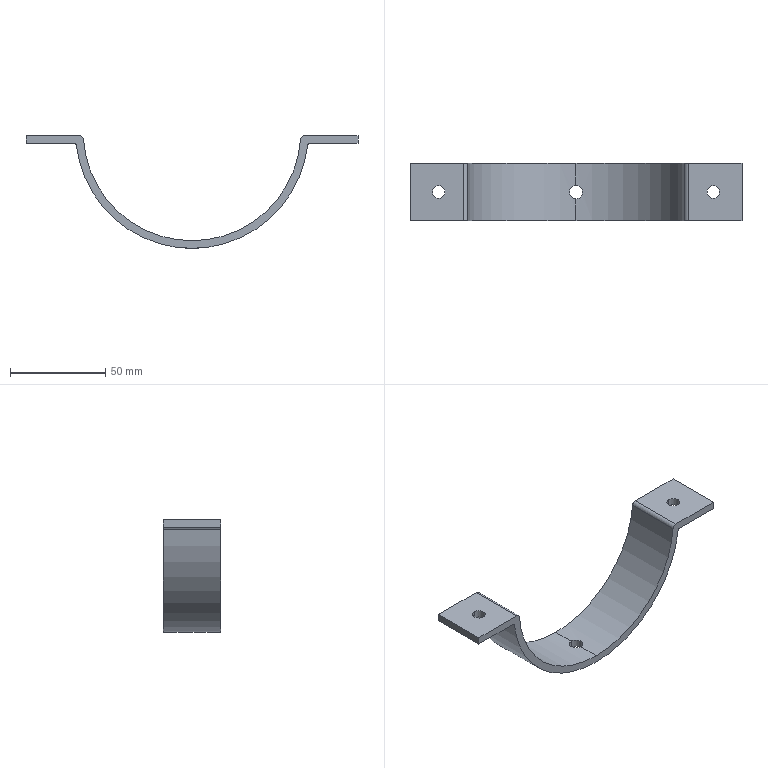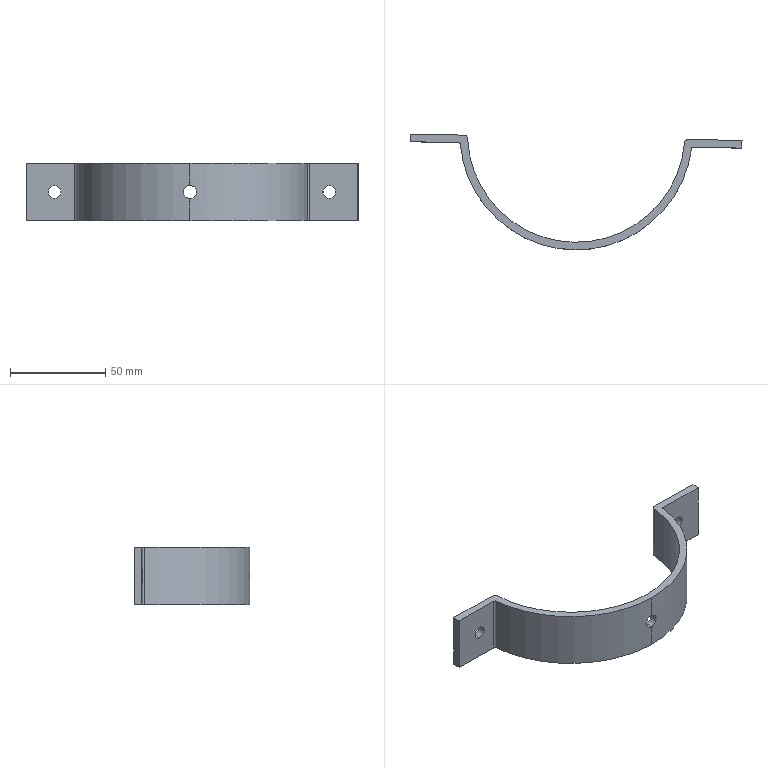Simulation study | abaqus
Set-up summary:
category,name,step,type,value,unit,region
solver,abaqus
solver,version,,,Abaqus/Standard 2020
units,not stated in the deck,,not stated
analysis,deck,,transient,transient
load_step,Step-1,Step-1,transient
load_step,requested,,,1
mesh,nodes,,,6600
mesh,elements,,,6768
element_type,B31,,beam,6768
load,load commands in deck,,count,4
bc,support commands in deck,,count,4
material,MATERIAL-1,,in results
material,MATERIAL-2,,in results
check,setup vs results,,match,"per instance, exact: element labels, types and connectivity; labels of the nodes the elements use; coordinates not compared"
Abaqus input file, long lists of numbers shortened, first 446 of 1701 lines:
*Heading
** Job name: Job-1 Model name: Model-2-Copy-Copy
** Generated by: Abaqus/CAE 2020
*Preprint, echo=NO, model=NO, history=NO, contact=NO
**
** PARTS
**
*Part, name=Part-1
*End Part
**
**
** ASSEMBLY
**
*Assembly, name=Assembly
**
*Instance, name=Part-1-1, part=Part-1
*Node
      1,        3710.,        3000.,        7130.
      2,        3710.,        2700.,        7430.
** (6598 more lines like these left out)
*Element, type=B31
1,   1, 481
2, 481, 482
** (6766 more lines like these left out)
*Nset, nset=Set-1
    7,    9,   10,   16,   27,   29,   30,   36,   47,   49,   50,   56,   72,   75,   77,   78
   92,   95,   97,   98,  112,  115,  117,  118,  132,  135,  137,  138,  152,  155,  157,  158
** (10 more lines like these left out)
*Elset, elset=Set-1
   81,   82,   83,  254,  255,  256,  363,  364,  365,  536,  537,  538,  645,  646,  647,  818
  819,  820, 1031, 1032, 1033, 1107, 1108, 1109, 1313, 1314, 1315, 1389, 1390, 1391, 1595, 1596
** (7 more lines like these left out)
*Nset, nset=Set-3
    7,    9,   10,   16,   27,   29,   30,   36,   47,   49,   50,   56,   72,   75,   77,   78
   92,   95,   97,   98,  112,  115,  117,  118,  132,  135,  137,  138,  152,  155,  157,  158
** (10 more lines like these left out)
*Elset, elset=Set-3
   81,   82,   83,  254,  255,  256,  363,  364,  365,  536,  537,  538,  645,  646,  647,  818
  819,  820, 1031, 1032, 1033, 1107, 1108, 1109, 1313, 1314, 1315, 1389, 1390, 1391, 1595, 1596
** (7 more lines like these left out)
*Nset, nset=Set-4
    7,    9,   10,   16,   27,   29,   30,   36,   47,   49,   50,   56,   72,   75,   77,   78
   92,   95,   97,   98,  112,  115,  117,  118,  132,  135,  137,  138,  152,  155,  157,  158
** (10 more lines like these left out)
*Elset, elset=Set-4
   81,   82,   83,  254,  255,  256,  363,  364,  365,  536,  537,  538,  645,  646,  647,  818
  819,  820, 1031, 1032, 1033, 1107, 1108, 1109, 1313, 1314, 1315, 1389, 1390, 1391, 1595, 1596
** (7 more lines like these left out)
*Nset, nset=Set-5
    7,    8,    9,   10,   16,   17,   18,   20,   27,   28,   29,   30,   36,   37,   38,   40
   47,   48,   49,   50,   56,   57,   58,   60,   72,   74,   75,   76,   77,   78,   79,   80
** (99 more lines like these left out)
*Elset, elset=Set-5
   74,   75,   76,   81,   82,   83,  209,  210,  211,  212,  213,  214,  215,  216,  217,  218
  219,  220,  221,  222,  223,  224,  225,  226,  227,  228,  229,  230,  231,  232,  233,  234
** (97 more lines like these left out)
*Nset, nset=Set-6
    8,    9,   16,   18,   28,   29,   36,   38,   48,   49,   56,   58,   74,   75,   78,   79
   94,   95,   98,   99,  114,  115,  118,  119,  134,  135,  138,  139,  154,  155,  158,  159
** (13 more lines like these left out)
*Elset, elset=Set-6
   77,   78,   79,   80,  257,  258,  259,  260,  359,  360,  361,  362,  539,  540,  541,  542
  641,  642,  643,  644,  821,  822,  823,  824, 1073, 1074, 1075, 1076, 1113, 1114, 1115, 1116
** (10 more lines like these left out)
*Nset, nset=Set-7
    1,    2,    3,    4,    5,    6,    7,    8,    9,   10,   11,   12,   13,   14,   15,   16
   17,   18,   19,   20,   21,   22,   23,   24,   25,   26,   27,   28,   29,   30,   31,   32
** (393 more lines like these left out)
*Elset, elset=Set-7
    5,    6,    7,    8,    9,   10,   11,   12,   13,   14,   15,   16,   17,   18,   19,   20
   21,   22,   23,   24,   25,   26,   27,   28,   29,   30,   31,   32,   33,   34,   35,   36
** (397 more lines like these left out)
*Nset, nset=Set-8
    1,    2,    4,    6,    8,    9,   11,   12,   13,   15,   16,   18,   21,   22,   24,   26
   28,   29,   31,   32,   33,   35,   36,   38,   41,   42,   44,   46,   48,   49,   51,   52
** (28 more lines like these left out)
*Elset, elset=Set-8
    1,    2,    3,    4,   77,   78,   79,   80,  138,  139,  140,  141,  205,  206,  207,  208
  257,  258,  259,  260,  267,  268,  269,  270,  283,  284,  285,  286,  359,  360,  361,  362
** (22 more lines like these left out)
*Nset, nset=Set-9
    1,    2,    3,    4,    5,    6,    7,    8,    9,   10,   11,   12,   13,   14,   15,   16
   17,   18,   19,   20,   21,   22,   23,   24,   25,   26,   27,   28,   29,   30,   31,   32
** (384 more lines like these left out)
*Elset, elset=Set-9
    5,    6,    7,    8,    9,   10,   11,   12,   13,   14,   15,   16,   17,   18,   19,   20
   21,   22,   23,   24,   25,   26,   27,   28,   29,   30,   31,   32,   33,   34,   35,   36
** (385 more lines like these left out)
*Nset, nset=Set-10
    1,    2,    4,    6,    8,    9,   11,   12,   13,   15,   16,   18,   21,   22,   24,   26
   28,   29,   31,   32,   33,   35,   36,   38,   41,   42,   44,   46,   48,   49,   51,   52
** (43 more lines like these left out)
*Elset, elset=Set-10
    1,    2,    3,    4,   77,   78,   79,   80,  138,  139,  140,  141,  205,  206,  207,  208
  257,  258,  259,  260,  267,  268,  269,  270,  283,  284,  285,  286,  359,  360,  361,  362
** (34 more lines like these left out)
*Nset, nset=Set-12
    1,    2,    3,    4,    5,    6,    7,    8,    9,   10,   11,   12,   13,   14,   15,   16
   17,   18,   19,   20,   21,   22,   23,   24,   25,   26,   27,   28,   29,   30,   31,   32
** (262 more lines like these left out)
*Elset, elset=Set-12
    1,    2,    3,    4,    5,    6,    7,   44,   45,   46,   47,   48,   49,   50,   51,   52
   53,   54,   55,   56,   57,   58,   59,   60,   61,   62,   63,   64,   65,   66,   67,   68
** (259 more lines like these left out)
*Nset, nset=Set-13
    1,    4,    8,   12,   13,   16,   21,   24,   28,   32,   33,   36,   41,   44,   48,   52
   53,   56,   61,   64,   68,   71,   74,   78,   81,   84,   88,   91,   94,   98,  101,  104
** (68 more lines like these left out)
*Elset, elset=Set-13
   11,   12,   13,   14,   15,   16,   17,   18,   19,   20,   21,   22,   23,   24,   25,   26
   27,   28,   29,   30,   31,   32,   33,   34,   35,   36,   37,   38,   39,   40,  142,  143
** (66 more lines like these left out)
*Nset, nset=Set-14
    1,    2,    3,    4,    5,    6,    7,    8,    9,   10,   11,   12,   13,   14,   15,   16
   18,   19,   21,   22,   23,   24,   25,   26,   27,   28,   29,   30,   31,   32,   33,   34
** (100 more lines like these left out)
*Elset, elset=Set-14
    1,    2,    3,    4,    8,    9,   10,   11,   12,   13,   14,   15,   16,   17,   18,   19
   20,   21,   22,   23,   24,   25,   26,   27,   28,   29,   30,   31,   32,   33,   34,   35
** (97 more lines like these left out)
*Nset, nset=Set-15
  121,  122,  123,  124,  125,  126,  127,  128,  129,  130,  131,  132,  133,  134,  135,  137
  138,  139,  141,  142,  143,  144,  145,  146,  147,  148,  149,  150,  151,  152,  153,  154
** (100 more lines like these left out)
*Elset, elset=Set-15
 1693, 1694, 1695, 1696, 1700, 1701, 1702, 1703, 1704, 1705, 1706, 1707, 1708, 1709, 1710, 1711
 1712, 1713, 1714, 1715, 1716, 1717, 1718, 1719, 1720, 1721, 1722, 1723, 1724, 1725, 1726, 1727
** (97 more lines like these left out)
*Orientation, name=Ori-1
1., 0., 0., 0., 1., 0.
1, 0.
** Region: (steel:Set-10), (Beam Orientation:Set-14), (Material Orientation:Picked)
*Elset, elset=_I1, internal
    1,    2,    3,    4,   77,   78,   79,   80,  138,  139,  140,  141,  205,  206,  207,  208
  257,  258,  259,  260,  267,  268,  269,  270,  283,  284,  285,  286,  359,  360,  361,  362
** (16 more lines like these left out)
** Section: steel  Profile: Profile-2
*Beam Section, elset=_I1, material=Material-2, temperature=GRADIENTS, section=BOX
40., 28., 2., 2., 2., 2.
1.,0.,0.
** Region: (Section-1:Set-9), (Beam Orientation:Set-12), (Material Orientation:Picked)
*Elset, elset=_I2, internal
    5,    6,    7,   44,   45,   46,   47,   48,   49,   50,   51,   52,   53,   54,   55,   56
   57,   58,   59,   60,   61,   62,   63,   64,   65,   66,   67,   68,   69,   70,   71,   72
** (223 more lines like these left out)
** Section: Section-1  Profile: Profile-1
*Beam Section, elset=_I2, material=Material-1, temperature=GRADIENTS, section=PIPE
55., 12.
0.,0.,-1.
** Region: (Section-1:Set-9), (Beam Orientation:Set-14), (Material Orientation:Picked)
*Elset, elset=_I3, internal
    8,    9,   10,   11,   12,   13,   14,   15,   16,   17,   18,   19,   20,   21,   22,   23
   24,   25,   26,   27,   28,   29,   30,   31,   32,   33,   34,   35,   36,   37,   38,   39
** (79 more lines like these left out)
** Section: Section-1  Profile: Profile-1
*Beam Section, elset=_I3, material=Material-1, temperature=GRADIENTS, section=PIPE
55., 12.
1.,0.,0.
** Region: (steel:Set-10), (Beam Orientation:Set-15), (Material Orientation:Picked)
*Elset, elset=_I4, internal
 1693, 1694, 1695, 1696, 1769, 1770, 1771, 1772, 1803, 1804, 1805, 1806, 1870, 1871, 1872, 1873
 1919, 1920, 1921, 1922, 1959, 1960, 1961, 1962, 1975, 1976, 1977, 1978, 2051, 2052, 2053, 2054
** (16 more lines like these left out)
** Section: steel  Profile: Profile-2
*Beam Section, elset=_I4, material=Material-2, temperature=GRADIENTS, section=BOX
40., 28., 2., 2., 2., 2.
0.,0.,-1.
** Region: (Section-1:Set-9), (Beam Orientation:Set-15), (Material Orientation:Picked)
*Elset, elset=_I5, internal
 1700, 1701, 1702, 1703, 1704, 1705, 1706, 1707, 1708, 1709, 1710, 1711, 1712, 1713, 1714, 1715
 1716, 1717, 1718, 1719, 1720, 1721, 1722, 1723, 1724, 1725, 1726, 1727, 1728, 1729, 1730, 1731
** (79 more lines like these left out)
** Section: Section-1  Profile: Profile-1
*Beam Section, elset=_I5, material=Material-1, temperature=GRADIENTS, section=PIPE
55., 12.
0.,0.,-1.
*End Instance
**
*Nset, nset=Set-1, instance=Part-1-1
  17,  20,  37,  40,  57,  60,  76,  80,  96, 100, 116, 120, 136, 140, 156, 160
 176, 180, 196, 200, 216, 220, 236, 240, 256, 260, 276, 280, 296, 300, 316, 320
** (1 more lines like these left out)
*Nset, nset=Set-2, instance=Part-1-1
  17,  20,  37,  40,  57,  60,  76,  80,  96, 100, 116, 120, 136, 140, 156, 160
 176, 180, 196, 200, 216, 220, 236, 240, 256, 260, 276, 280, 296, 300, 316, 320
** (1 more lines like these left out)
*Nset, nset=Set-58, instance=Part-1-1
   7,  10,  27,  30,  47,  50,  72,  77,  92,  97, 112, 117, 132, 137, 152, 157
 172, 177, 192, 197, 212, 217, 232, 237, 252, 257, 272, 277, 292, 297, 312, 317
** (1 more lines like these left out)
*Nset, nset=Set-59, instance=Part-1-1
   1,   2,   3,   4,   5,   6,   7,   8,   9,  10,  11,  12,  13,  14,  15,  16
  18,  19,  21,  22,  23,  24,  25,  26,  27,  28,  29,  30,  31,  32,  33,  34
** (25 more lines like these left out)
*Nset, nset=m_Set-3, instance=Part-1-1
 205, 223, 243, 305
*Nset, nset=m_Set-6, instance=Part-1-1
 207, 230, 250, 307
*Nset, nset=m_Set-8, instance=Part-1-1
 212, 237, 257, 312
*Nset, nset=m_Set-10, instance=Part-1-1
  72, 412
*Nset, nset=m_Set-12, instance=Part-1-1
  77, 417, 447, 467
*Nset, nset=m_Set-14, instance=Part-1-1
 450, 470
*Nset, nset=m_Set-16, instance=Part-1-1
 137, 172, 297, 352
*Nset, nset=m_Set-18, instance=Part-1-1
  50, 430
*Nset, nset=m_Set-20, instance=Part-1-1
  47, 117, 377, 427
*Nset, nset=m_Set-22, instance=Part-1-1
 112, 372
*Nset, nset=m_Set-24, instance=Part-1-1
 157, 192, 277, 332
*Nset, nset=m_Set-26, instance=Part-1-1
 227, 247
*Nset, nset=m_Set-28, instance=Part-1-1
  45, 110, 370, 425
*Nset, nset=m_Set-30, instance=Part-1-1
   5,  25,  90, 390
*Nset, nset=m_Set-32, instance=Part-1-1
  63, 403, 454, 474
*Nset, nset=m_Set-34, instance=Part-1-1
  70, 410, 445, 465
*Nset, nset=m_Set-36, instance=Part-1-1
 170, 350
*Nset, nset=m_Set-38, instance=Part-1-1
 210, 310
*Nset, nset=m_Set-40, instance=Part-1-1
 130, 167, 290, 347
*Nset, nset=m_Set-42, instance=Part-1-1
 127, 287
*Nset, nset=m_Set-44, instance=Part-1-1
  59, 439
*Nset, nset=m_Set-46, instance=Part-1-1
  54, 103, 363, 434
*Nset, nset=m_Set-48, instance=Part-1-1
 143, 185, 263, 325
*Nset, nset=m_Set-50, instance=Part-1-1
 203, 303
*Nset, nset=m_Set-52, instance=Part-1-1
 225, 245
*Nset, nset=m_Set-54, instance=Part-1-1
 459, 479
*Nset, nset=m_Set-56, instance=Part-1-1
 123, 165, 283, 345
*Nset, nset=s_Set-3, instance=Part-1-1
 385,
*Nset, nset=s_Set-5, instance=Part-1-1
  85, 385
*Nset, nset=s_Set-6, instance=Part-1-1
  87, 387
*Nset, nset=s_Set-8, instance=Part-1-1
  92, 392
*Nset, nset=s_Set-10, instance=Part-1-1
 217, 317
*Nset, nset=s_Set-12, instance=Part-1-1
 197, 337
*Nset, nset=s_Set-14, instance=Part-1-1
 177, 357
*Nset, nset=s_Set-16, instance=Part-1-1
 10, 30
*Nset, nset=s_Set-18, instance=Part-1-1
 132, 292
*Nset, nset=s_Set-20, instance=Part-1-1
 152, 272
*Nset, nset=s_Set-22, instance=Part-1-1
 232, 252
*Nset, nset=s_Set-24, instance=Part-1-1
   7,  27,  97, 397
*Nset, nset=s_Set-26, instance=Part-1-1
 107, 367
*Nset, nset=s_Set-28, instance=Part-1-1
 147, 267
*Nset, nset=s_Set-30, instance=Part-1-1
 150, 187, 270, 327
*Nset, nset=s_Set-32, instance=Part-1-1
 183, 323
*Nset, nset=s_Set-34, instance=Part-1-1
 190, 330
*Nset, nset=s_Set-36, instance=Part-1-1
 443, 463
*Nset, nset=s_Set-38, instance=Part-1-1
  67, 407
*Nset, nset=s_Set-40, instance=Part-1-1
  3, 23
*Nset, nset=s_Set-42, instance=Part-1-1
  43, 423
*Nset, nset=s_Set-44, instance=Part-1-1
 125, 285
*Nset, nset=s_Set-46, instance=Part-1-1
 145, 265
*Nset, nset=s_Set-48, instance=Part-1-1
  14,  34,  83, 383
*Nset, nset=s_Set-50, instance=Part-1-1
  65, 405
*Nset, nset=s_Set-52, instance=Part-1-1
 105, 365
*Nset, nset=s_Set-54, instance=Part-1-1
 163, 343
*Nset, nset=s_Set-56, instance=Part-1-1
 19, 39
*Elset, elset=_m_Surf-1_, internal, instance=Part-1-1, generate
 1923,  1952,     1
*Surface, type=ELEMENT, name=m_Surf-1
_m_Surf-1_,
*Elset, elset=_m_Surf-3_, internal, instance=Part-1-1, generate
 5025,  5054,     1
*Surface, type=ELEMENT, name=m_Surf-3
_m_Surf-3_,
*Elset, elset=_m_Surf-5_, internal, instance=Part-1-1, generate
 1807,  1836,     1
*Surface, type=ELEMENT, name=m_Surf-5
_m_Surf-5_,
*Elset, elset=_m_Surf-7_, internal, instance=Part-1-1, generate
 4909,  4938,     1
*Surface, type=ELEMENT, name=m_Surf-7
_m_Surf-7_,
*Elset, elset=_m_Surf-9_, internal, instance=Part-1-1, generate
 1703,  1732,     1
*Surface, type=ELEMENT, name=m_Surf-9
_m_Surf-9_,
*Elset, elset=_m_Surf-11_, internal, instance=Part-1-1, generate
 4805,  4834,     1
*Surface, type=ELEMENT, name=m_Surf-11
_m_Surf-11_,
*Elset, elset=_m_Surf-13_, internal, instance=Part-1-1, generate
 1985,  2014,     1
*Surface, type=ELEMENT, name=m_Surf-13
_m_Surf-13_,
*Elset, elset=_m_Surf-15_, internal, instance=Part-1-1, generate
 4523,  4552,     1
*Surface, type=ELEMENT, name=m_Surf-15
_m_Surf-15_,
*Elset, elset=_m_Surf-17_, internal, instance=Part-1-1, generate
 3395,  3424,     1
*Surface, type=ELEMENT, name=m_Surf-17
_m_Surf-17_,
*Elset, elset=_m_Surf-19_, internal, instance=Part-1-1, generate
 4241,  4270,     1
*Surface, type=ELEMENT, name=m_Surf-19
_m_Surf-19_,
*Elset, elset=_m_Surf-21_, internal, instance=Part-1-1, generate
 706,  735,    1
*Surface, type=ELEMENT, name=m_Surf-21
_m_Surf-21_,
*Elset, elset=_m_Surf-23_, internal, instance=Part-1-1, generate
 424,  453,    1
*Surface, type=ELEMENT, name=m_Surf-23
_m_Surf-23_,
*Elset, elset=_m_Surf-25_, internal, instance=Part-1-1, generate
 1641,  1670,     1
*Surface, type=ELEMENT, name=m_Surf-25
_m_Surf-25_,
*Elset, elset=_m_Surf-27_, internal, instance=Part-1-1, generate
 773,  802,    1
*Surface, type=ELEMENT, name=m_Surf-27
_m_Surf-27_,
*Elset, elset=_m_Surf-29_, internal, instance=Part-1-1, generate
 1525,  1554,     1
*Surface, type=ELEMENT, name=m_Surf-29
_m_Surf-29_,
*Elset, elset=_m_Surf-31_, internal, instance=Part-1-1, generate
 575,  604,    1
*Surface, type=ELEMENT, name=m_Surf-31
_m_Surf-31_,
*Elset, elset=_m_Surf-33_, internal, instance=Part-1-1, generate
 1421,  1450,     1
*Surface, type=ELEMENT, name=m_Surf-33
_m_Surf-33_,
*Elset, elset=_m_Surf-35_, internal, instance=Part-1-1, generate
 1139,  1168,     1
*Surface, type=ELEMENT, name=m_Surf-35
_m_Surf-35_,
*Elset, elset=_m_Surf-37_, internal, instance=Part-1-1, generate
 5651,  5680,     1
*Surface, type=ELEMENT, name=m_Surf-37
_m_Surf-37_,
*Elset, elset=_m_Surf-39_, internal, instance=Part-1-1, generate
 6346,  6375,     1
*Surface, type=ELEMENT, name=m_Surf-39
_m_Surf-39_,
*Elset, elset=_m_Surf-41_, internal, instance=Part-1-1, generate
 961,  990,    1
*Surface, type=ELEMENT, name=m_Surf-41
_m_Surf-41_,
*Elset, elset=_m_Surf-43_, internal, instance=Part-1-1, generate
 6215,  6244,     1
*Surface, type=ELEMENT, name=m_Surf-43
_m_Surf-43_,
*Elset, elset=_m_Surf-45_, internal, instance=Part-1-1, generate
 1077,  1106,     1
*Surface, type=ELEMENT, name=m_Surf-45
_m_Surf-45_,
*Elset, elset=_m_Surf-47_, internal, instance=Part-1-1, generate
 6413,  6442,     1
*Surface, type=ELEMENT, name=m_Surf-47
_m_Surf-47_,
*Elset, elset=_m_Surf-49_, internal, instance=Part-1-1, generate
 1243,  1272,     1
*Surface, type=ELEMENT, name=m_Surf-49
_m_Surf-49_,
*Elset, elset=_m_Surf-51_, internal, instance=Part-1-1, generate
 293,  322,    1
*Surface, type=ELEMENT, name=m_Surf-51
_m_Surf-51_,
*Elset, elset=_m_Surf-53_, internal, instance=Part-1-1, generate
 1359,  1388,     1
*Surface, type=ELEMENT, name=m_Surf-53
_m_Surf-53_,
*Elset, elset=_m_Surf-55_, internal, instance=Part-1-1, generate
 491,  520,    1
*Surface, type=ELEMENT, name=m_Surf-55
_m_Surf-55_,
*Elset, elset=_m_Surf-57_, internal, instance=Part-1-1, generate
  991,  1017,     1
*Surface, type=ELEMENT, name=m_Surf-57
_m_Surf-57_,
*Elset, elset=_m_Surf-59_, internal, instance=Part-1-1, generate
 4430,  4456,     1
*Surface, type=ELEMENT, name=m_Surf-59
_m_Surf-59_,
*Elset, elset=_m_Surf-61_, internal, instance=Part-1-1, generate
 4743,  4772,     1
*Surface, type=ELEMENT, name=m_Surf-61
_m_Surf-61_,
*Elset, elset=_m_Surf-63_, internal, instance=Part-1-1, generate
 4461,  4490,     1
*Surface, type=ELEMENT, name=m_Surf-63
_m_Surf-63_,
*Elset, elset=_m_Surf-65_, internal, instance=Part-1-1, generate
 3615,  3644,     1
*Surface, type=ELEMENT, name=m_Surf-65
_m_Surf-65_,
*Elset, elset=_m_Surf-67_, internal, instance=Part-1-1, generate
 2935,  2964,     1
*Surface, type=ELEMENT, name=m_Surf-67
_m_Surf-67_,
*Elset, elset=_m_Surf-69_, internal, instance=Part-1-1, generate
 2205,  2234,     1
*Surface, type=ELEMENT, name=m_Surf-69
_m_Surf-69_,
*Elset, elset=_m_Surf-71_, internal, instance=Part-1-1, generate
 4627,  4656,     1
Last 806 lines:
_s_Surf-103_,
*Elset, elset=_s_Surf-105_, internal, instance=Part-1-1, generate
 6033,  6059,     1
*Surface, type=ELEMENT, name=s_Surf-105
_s_Surf-105_,
*Elset, elset=_s_Surf-107_, internal, instance=Part-1-1, generate
 3995,  4021,     1
*Surface, type=ELEMENT, name=s_Surf-107
_s_Surf-107_,
*Elset, elset=_s_Surf-109_, internal, instance=Part-1-1, generate
 5160,  5186,     1
*Surface, type=ELEMENT, name=s_Surf-109
_s_Surf-109_,
*Elset, elset=_s_Surf-111_, internal, instance=Part-1-1, generate
 1494,  1520,     1
*Surface, type=ELEMENT, name=s_Surf-111
_s_Surf-111_,
*Elset, elset=_s_Surf-113_, internal, instance=Part-1-1, generate
 3713,  3739,     1
*Surface, type=ELEMENT, name=s_Surf-113
_s_Surf-113_,
*Elset, elset=_s_Surf-116_, internal, instance=Part-1-1, generate
 6100,  6126,     1
*Surface, type=ELEMENT, name=s_Surf-116
_s_Surf-116_,
*Elset, elset=_s_Surf-118_, internal, instance=Part-1-1, generate
 1610,  1636,     1
*Surface, type=ELEMENT, name=s_Surf-118
_s_Surf-118_,
*Elset, elset=_s_Surf-120_, internal, instance=Part-1-1, generate
 2119,  2145,     1
*Surface, type=ELEMENT, name=s_Surf-120
_s_Surf-120_,
*Elset, elset=_s_Surf-122_, internal, instance=Part-1-1, generate
 5969,  5995,     1
*Surface, type=ELEMENT, name=s_Surf-122
_s_Surf-122_,
*Elset, elset=_s_Surf-124_, internal, instance=Part-1-1, generate
 3431,  3457,     1
*Surface, type=ELEMENT, name=s_Surf-124
_s_Surf-124_,
*Elset, elset=_s_Surf-126_, internal, instance=Part-1-1, generate
 5123,  5149,     1
*Surface, type=ELEMENT, name=s_Surf-126
_s_Surf-126_,
*Elset, elset=_s_Surf-128_, internal, instance=Part-1-1, generate
 4277,  4303,     1
*Surface, type=ELEMENT, name=s_Surf-128
_s_Surf-128_,
*Elset, elset=_s_Surf-130_, internal, instance=Part-1-1, generate
 5405,  5431,     1
*Surface, type=ELEMENT, name=s_Surf-130
_s_Surf-130_,
*Elset, elset=_s_Surf-132_, internal, instance=Part-1-1, generate
 3186,  3212,     1
*Surface, type=ELEMENT, name=s_Surf-132
_s_Surf-132_,
*Elset, elset=_s_Surf-134_, internal, instance=Part-1-1, generate
 5687,  5713,     1
*Surface, type=ELEMENT, name=s_Surf-134
_s_Surf-134_,
*Elset, elset=_s_Surf-136_, internal, instance=Part-1-1, generate
 4314,  4340,     1
*Surface, type=ELEMENT, name=s_Surf-136
_s_Surf-136_,
*Elset, elset=_s_Surf-138_, internal, instance=Part-1-1, generate
 6597,  6623,     1
*Surface, type=ELEMENT, name=s_Surf-138
_s_Surf-138_,
*Elset, elset=_s_Surf-140_, internal, instance=Part-1-1, generate
 2340,  2366,     1
*Surface, type=ELEMENT, name=s_Surf-140
_s_Surf-140_,
*Elset, elset=_s_Surf-142_, internal, instance=Part-1-1, generate
 2303,  2329,     1
*Surface, type=ELEMENT, name=s_Surf-142
_s_Surf-142_,
*Elset, elset=_s_Surf-144_, internal, instance=Part-1-1, generate
 111,  137,    1
*Surface, type=ELEMENT, name=s_Surf-144
_s_Surf-144_,
*Elset, elset=_s_Surf-146_, internal, instance=Part-1-1, generate
 4032,  4058,     1
*Surface, type=ELEMENT, name=s_Surf-146
_s_Surf-146_,
*Elset, elset=_s_Surf-148_, internal, instance=Part-1-1, generate
 5724,  5750,     1
*Surface, type=ELEMENT, name=s_Surf-148
_s_Surf-148_,
*Elset, elset=_s_Surf-150_, internal, instance=Part-1-1, generate
 2622,  2648,     1
*Surface, type=ELEMENT, name=s_Surf-150
_s_Surf-150_,
*Elset, elset=_s_Surf-152_, internal, instance=Part-1-1, generate
 6664,  6690,     1
*Surface, type=ELEMENT, name=s_Surf-152
_s_Surf-152_,
*Elset, elset=_s_Surf-154_, internal, instance=Part-1-1, generate
 4657,  4683,     1
*Surface, type=ELEMENT, name=s_Surf-154
_s_Surf-154_,
*Elset, elset=_s_Surf-156_, internal, instance=Part-1-1, generate
 5558,  5584,     1
*Surface, type=ELEMENT, name=s_Surf-156
_s_Surf-156_,
*Elset, elset=_s_Surf-158_, internal, instance=Part-1-1, generate
 2174,  2200,     1
*Surface, type=ELEMENT, name=s_Surf-158
_s_Surf-158_,
*Elset, elset=_s_Surf-160_, internal, instance=Part-1-1, generate
 2585,  2611,     1
*Surface, type=ELEMENT, name=s_Surf-160
_s_Surf-160_,
*Elset, elset=_s_Surf-162_, internal, instance=Part-1-1, generate
 178,  204,    1
*Surface, type=ELEMENT, name=s_Surf-162
_s_Surf-162_,
*Elset, elset=_s_Surf-164_, internal, instance=Part-1-1, generate
 3750,  3776,     1
*Surface, type=ELEMENT, name=s_Surf-164
_s_Surf-164_,
*Elset, elset=_s_Surf-166_, internal, instance=Part-1-1, generate
 1212,  1238,     1
*Surface, type=ELEMENT, name=s_Surf-166
_s_Surf-166_,
*Elset, elset=_s_Surf-168_, internal, instance=Part-1-1, generate
 2487,  2516,     1
*Surface, type=ELEMENT, name=s_Surf-168
_s_Surf-168_,
*Elset, elset=_s_Surf-170_, internal, instance=Part-1-1, generate
 4179,  4208,     1
*Surface, type=ELEMENT, name=s_Surf-170
_s_Surf-170_,
*Elset, elset=_s_Surf-172_, internal, instance=Part-1-1, generate
 4063,  4092,     1
*Surface, type=ELEMENT, name=s_Surf-172
_s_Surf-172_,
*Elset, elset=_s_Surf-174_, internal, instance=Part-1-1, generate
 2371,  2400,     1
*Surface, type=ELEMENT, name=s_Surf-174
_s_Surf-174_,
*Elset, elset=_s_Surf-176_, internal, instance=Part-1-1, generate
 3959,  3988,     1
*Surface, type=ELEMENT, name=s_Surf-176
_s_Surf-176_,
*Elset, elset=_s_Surf-178_, internal, instance=Part-1-1, generate
 2267,  2296,     1
*Surface, type=ELEMENT, name=s_Surf-178
_s_Surf-178_,
*Elset, elset=_s_Surf-180_, internal, instance=Part-1-1, generate
 3677,  3706,     1
*Surface, type=ELEMENT, name=s_Surf-180
_s_Surf-180_,
*Elset, elset=_s_Surf-182_, internal, instance=Part-1-1, generate
 2549,  2578,     1
*Surface, type=ELEMENT, name=s_Surf-182
_s_Surf-182_,
*Elset, elset=_s_Surf-184_, internal, instance=Part-1-1, generate
 3113,  3142,     1
*Surface, type=ELEMENT, name=s_Surf-184
_s_Surf-184_,
*Elset, elset=_s_Surf-186_, internal, instance=Part-1-1, generate
 2831,  2860,     1
*Surface, type=ELEMENT, name=s_Surf-186
_s_Surf-186_,
*Elset, elset=_s_Surf-188_, internal, instance=Part-1-1, generate
 6064,  6093,     1
*Surface, type=ELEMENT, name=s_Surf-188
_s_Surf-188_,
*Elset, elset=_s_Surf-190_, internal, instance=Part-1-1, generate
 142,  171,    1
*Surface, type=ELEMENT, name=s_Surf-190
_s_Surf-190_,
*Surface, type=NODE, name=m_Set-3_CNS_, internal
m_Set-3, 1.
*Surface, type=NODE, name=s_Set-5_CNS_, internal
s_Set-5, 1.
*Surface, type=NODE, name=m_Set-6_CNS_, internal
m_Set-6, 1.
*Surface, type=NODE, name=s_Set-6_CNS_, internal
s_Set-6, 1.
*Surface, type=NODE, name=m_Set-8_CNS_, internal
m_Set-8, 1.
*Surface, type=NODE, name=s_Set-8_CNS_, internal
s_Set-8, 1.
*Surface, type=NODE, name=m_Set-10_CNS_, internal
m_Set-10, 1.
*Surface, type=NODE, name=s_Set-10_CNS_, internal
s_Set-10, 1.
*Surface, type=NODE, name=m_Set-12_CNS_, internal
m_Set-12, 1.
*Surface, type=NODE, name=s_Set-12_CNS_, internal
s_Set-12, 1.
*Surface, type=NODE, name=m_Set-14_CNS_, internal
m_Set-14, 1.
*Surface, type=NODE, name=s_Set-14_CNS_, internal
s_Set-14, 1.
*Surface, type=NODE, name=m_Set-16_CNS_, internal
m_Set-16, 1.
*Surface, type=NODE, name=s_Set-16_CNS_, internal
s_Set-16, 1.
*Surface, type=NODE, name=m_Set-18_CNS_, internal
m_Set-18, 1.
*Surface, type=NODE, name=s_Set-18_CNS_, internal
s_Set-18, 1.
*Surface, type=NODE, name=m_Set-20_CNS_, internal
m_Set-20, 1.
*Surface, type=NODE, name=s_Set-20_CNS_, internal
s_Set-20, 1.
*Surface, type=NODE, name=m_Set-22_CNS_, internal
m_Set-22, 1.
*Surface, type=NODE, name=s_Set-22_CNS_, internal
s_Set-22, 1.
*Surface, type=NODE, name=m_Set-24_CNS_, internal
m_Set-24, 1.
*Surface, type=NODE, name=s_Set-24_CNS_, internal
s_Set-24, 1.
*Surface, type=NODE, name=m_Set-26_CNS_, internal
m_Set-26, 1.
*Surface, type=NODE, name=s_Set-26_CNS_, internal
s_Set-26, 1.
*Surface, type=NODE, name=m_Set-28_CNS_, internal
m_Set-28, 1.
*Surface, type=NODE, name=s_Set-28_CNS_, internal
s_Set-28, 1.
*Surface, type=NODE, name=m_Set-30_CNS_, internal
m_Set-30, 1.
*Surface, type=NODE, name=s_Set-30_CNS_, internal
s_Set-30, 1.
*Surface, type=NODE, name=m_Set-32_CNS_, internal
m_Set-32, 1.
*Surface, type=NODE, name=s_Set-32_CNS_, internal
s_Set-32, 1.
*Surface, type=NODE, name=m_Set-34_CNS_, internal
m_Set-34, 1.
*Surface, type=NODE, name=s_Set-34_CNS_, internal
s_Set-34, 1.
*Surface, type=NODE, name=m_Set-36_CNS_, internal
m_Set-36, 1.
*Surface, type=NODE, name=s_Set-36_CNS_, internal
s_Set-36, 1.
*Surface, type=NODE, name=m_Set-38_CNS_, internal
m_Set-38, 1.
*Surface, type=NODE, name=s_Set-38_CNS_, internal
s_Set-38, 1.
*Surface, type=NODE, name=m_Set-40_CNS_, internal
m_Set-40, 1.
*Surface, type=NODE, name=s_Set-40_CNS_, internal
s_Set-40, 1.
*Surface, type=NODE, name=m_Set-42_CNS_, internal
m_Set-42, 1.
*Surface, type=NODE, name=s_Set-42_CNS_, internal
s_Set-42, 1.
*Surface, type=NODE, name=m_Set-44_CNS_, internal
m_Set-44, 1.
*Surface, type=NODE, name=s_Set-44_CNS_, internal
s_Set-44, 1.
*Surface, type=NODE, name=m_Set-46_CNS_, internal
m_Set-46, 1.
*Surface, type=NODE, name=s_Set-46_CNS_, internal
s_Set-46, 1.
*Surface, type=NODE, name=m_Set-48_CNS_, internal
m_Set-48, 1.
*Surface, type=NODE, name=s_Set-48_CNS_, internal
s_Set-48, 1.
*Surface, type=NODE, name=m_Set-50_CNS_, internal
m_Set-50, 1.
*Surface, type=NODE, name=s_Set-50_CNS_, internal
s_Set-50, 1.
*Surface, type=NODE, name=m_Set-52_CNS_, internal
m_Set-52, 1.
*Surface, type=NODE, name=s_Set-52_CNS_, internal
s_Set-52, 1.
*Surface, type=NODE, name=m_Set-54_CNS_, internal
m_Set-54, 1.
*Surface, type=NODE, name=s_Set-54_CNS_, internal
s_Set-54, 1.
*Surface, type=NODE, name=m_Set-56_CNS_, internal
m_Set-56, 1.
*Surface, type=NODE, name=s_Set-56_CNS_, internal
s_Set-56, 1.
** Constraint: Constraint-1
*Tie, name=Constraint-1, adjust=yes
s_Surf-170, m_Surf-170
** Constraint: Constraint-2
*Tie, name=Constraint-2, adjust=yes
s_Surf-168, m_Surf-168
** Constraint: Constraint-3
*Tie, name=Constraint-3, adjust=yes
s_Surf-172, m_Surf-172
** Constraint: Constraint-4
*Tie, name=Constraint-4, adjust=yes
s_Surf-174, m_Surf-174
** Constraint: Constraint-5
*Tie, name=Constraint-5, adjust=yes
s_Surf-176, m_Surf-176
** Constraint: Constraint-6
*Tie, name=Constraint-6, adjust=yes
s_Surf-178, m_Surf-178
** Constraint: Constraint-7
*Tie, name=Constraint-7, adjust=yes
s_Surf-180, m_Surf-180
** Constraint: Constraint-8
*Tie, name=Constraint-8, adjust=yes
s_Surf-182, m_Surf-182
** Constraint: Constraint-9
*Tie, name=Constraint-9, adjust=yes
s_Surf-184, m_Surf-184
** Constraint: Constraint-10
*Tie, name=Constraint-10, adjust=yes
s_Surf-186, m_Surf-186
** Constraint: Constraint-11
*Tie, name=Constraint-11, adjust=yes
s_Surf-188, m_Surf-188
** Constraint: Constraint-12
*Tie, name=Constraint-12, adjust=yes
s_Surf-190, m_Surf-190
** Constraint: Constraint-13-node
*Tie, name=Constraint-13-node, adjust=yes
s_Set-5_CNS_, m_Set-3_CNS_
** Constraint: Constraint-14
*Tie, name=Constraint-14, adjust=yes
s_Set-6_CNS_, m_Set-6_CNS_
** Constraint: Constraint-15
*Tie, name=Constraint-15, adjust=yes
s_Set-8_CNS_, m_Set-8_CNS_
** Constraint: Constraint-16
*Tie, name=Constraint-16, adjust=yes
s_Set-10_CNS_, m_Set-10_CNS_
** Constraint: Constraint-17
*Tie, name=Constraint-17, adjust=yes
s_Set-12_CNS_, m_Set-12_CNS_
** Constraint: Constraint-18
*Tie, name=Constraint-18, adjust=yes
s_Set-14_CNS_, m_Set-14_CNS_
** Constraint: Constraint-19
*Tie, name=Constraint-19, adjust=yes
s_Set-16_CNS_, m_Set-16_CNS_
** Constraint: Constraint-20
*Tie, name=Constraint-20, adjust=yes
s_Set-18_CNS_, m_Set-18_CNS_
** Constraint: Constraint-21
*Tie, name=Constraint-21, adjust=yes
s_Set-20_CNS_, m_Set-20_CNS_
** Constraint: Constraint-22
*Tie, name=Constraint-22, adjust=yes
s_Set-22_CNS_, m_Set-22_CNS_
** Constraint: Constraint-23
*Tie, name=Constraint-23, adjust=yes
s_Set-24_CNS_, m_Set-24_CNS_
** Constraint: Constraint-24
*Tie, name=Constraint-24, adjust=yes
s_Set-26_CNS_, m_Set-26_CNS_
** Constraint: Constraint-25
*Tie, name=Constraint-25, adjust=yes
s_Set-28_CNS_, m_Set-28_CNS_
** Constraint: Constraint-26
*Tie, name=Constraint-26, adjust=yes
s_Set-30_CNS_, m_Set-30_CNS_
** Constraint: Constraint-27
*Tie, name=Constraint-27, adjust=yes
s_Set-32_CNS_, m_Set-32_CNS_
** Constraint: Constraint-28
*Tie, name=Constraint-28, adjust=yes
s_Set-34_CNS_, m_Set-34_CNS_
** Constraint: Constraint-29
*Tie, name=Constraint-29, adjust=yes
s_Set-36_CNS_, m_Set-36_CNS_
** Constraint: Constraint-30
*Tie, name=Constraint-30, adjust=yes
s_Set-38_CNS_, m_Set-38_CNS_
** Constraint: Constraint-31
*Tie, name=Constraint-31, adjust=yes
s_Set-40_CNS_, m_Set-40_CNS_
** Constraint: Constraint-32
*Tie, name=Constraint-32, adjust=yes
s_Set-42_CNS_, m_Set-42_CNS_
** Constraint: Constraint-33
*Tie, name=Constraint-33, adjust=yes
s_Set-44_CNS_, m_Set-44_CNS_
** Constraint: Constraint-34
*Tie, name=Constraint-34, adjust=yes
s_Set-46_CNS_, m_Set-46_CNS_
** Constraint: Constraint-35
*Tie, name=Constraint-35, adjust=yes
s_Set-48_CNS_, m_Set-48_CNS_
** Constraint: Constraint-36
*Tie, name=Constraint-36, adjust=yes
s_Set-50_CNS_, m_Set-50_CNS_
** Constraint: Constraint-37
*Tie, name=Constraint-37, adjust=yes
s_Set-52_CNS_, m_Set-52_CNS_
** Constraint: Constraint-38
*Tie, name=Constraint-38, adjust=yes
s_Set-54_CNS_, m_Set-54_CNS_
** Constraint: Constraint-39
*Tie, name=Constraint-39, adjust=yes
s_Set-56_CNS_, m_Set-56_CNS_
** Constraint: Constraint-40
*Tie, name=Constraint-40, adjust=yes
s_Surf-25, m_Surf-25
** Constraint: Constraint-41
*Tie, name=Constraint-41, adjust=yes
s_Surf-27, m_Surf-27
** Constraint: Constraint-42
*Tie, name=Constraint-42, adjust=yes
s_Surf-29, m_Surf-29
** Constraint: Constraint-43
*Tie, name=Constraint-43, adjust=yes
s_Surf-31, m_Surf-31
** Constraint: Constraint-44
*Tie, name=Constraint-44, adjust=yes
s_Surf-33, m_Surf-33
** Constraint: Constraint-45
*Tie, name=Constraint-45, adjust=yes
s_Surf-35, m_Surf-35
** Constraint: Constraint-46
*Tie, name=Constraint-46, adjust=yes
s_Surf-37, m_Surf-37
** Constraint: Constraint-47
*Tie, name=Constraint-47, adjust=yes
s_Surf-39, m_Surf-39
** Constraint: Constraint-48
*Tie, name=Constraint-48, adjust=yes
s_Surf-41, m_Surf-41
** Constraint: Constraint-49
*Tie, name=Constraint-49, adjust=yes
s_Surf-43, m_Surf-43
** Constraint: Constraint-50
*Tie, name=Constraint-50, adjust=yes
s_Surf-45, m_Surf-45
** Constraint: Constraint-51
*Tie, name=Constraint-51, adjust=yes
s_Surf-47, m_Surf-47
** Constraint: Constraint-52
*Tie, name=Constraint-52, adjust=yes
s_Surf-49, m_Surf-49
** Constraint: Constraint-53
*Tie, name=Constraint-53, adjust=yes
s_Surf-51, m_Surf-51
** Constraint: Constraint-54
*Tie, name=Constraint-54, adjust=yes
s_Surf-53, m_Surf-53
** Constraint: Constraint-55
*Tie, name=Constraint-55, adjust=yes
s_Surf-55, m_Surf-55
** Constraint: Constraint-56
*Tie, name=Constraint-56, adjust=yes
s_Surf-57, m_Surf-57
** Constraint: Constraint-57
*Tie, name=Constraint-57, adjust=yes
s_Surf-59, m_Surf-59
** Constraint: Constraint-58
*Tie, name=Constraint-58, adjust=yes
s_Surf-61, m_Surf-61
** Constraint: Constraint-59
*Tie, name=Constraint-59, adjust=yes
s_Surf-63, m_Surf-63
** Constraint: Constraint-60
*Tie, name=Constraint-60, adjust=yes
s_Surf-65, m_Surf-65
** Constraint: Constraint-61
*Tie, name=Constraint-61, adjust=yes
s_Surf-67, m_Surf-67
** Constraint: Constraint-62
*Tie, name=Constraint-62, adjust=yes
s_Surf-69, m_Surf-69
** Constraint: Constraint-63
*Tie, name=Constraint-63, adjust=yes
s_Surf-71, m_Surf-71
** Constraint: Constraint-64
*Tie, name=Constraint-64, adjust=yes
s_Surf-73, m_Surf-73
** Constraint: Constraint-65
*Tie, name=Constraint-65, adjust=yes
s_Surf-75, m_Surf-75
** Constraint: Constraint-66
*Tie, name=Constraint-66, adjust=yes
s_Surf-77, m_Surf-77
** Constraint: Constraint-67
*Tie, name=Constraint-67, adjust=yes
s_Surf-79, m_Surf-79
** Constraint: Constraint-68
*Tie, name=Constraint-68, adjust=yes
s_Surf-81, m_Surf-81
** Constraint: Constraint-69
*Tie, name=Constraint-69, adjust=yes
s_Surf-83, m_Surf-83
** Constraint: Constraint-70
*Tie, name=Constraint-70, adjust=yes
s_Surf-85, m_Surf-85
** Constraint: Constraint-71
*Tie, name=Constraint-71, adjust=yes
s_Surf-87, m_Surf-87
** Constraint: Constraint-72
*Tie, name=Constraint-72, adjust=yes
s_Surf-89, m_Surf-89
** Constraint: Constraint-73
*Tie, name=Constraint-73, adjust=yes
s_Surf-91, m_Surf-91
** Constraint: Constraint-74
*Tie, name=Constraint-74, adjust=yes
s_Surf-93, m_Surf-93
** Constraint: Constraint-75
*Tie, name=Constraint-75, adjust=yes
s_Surf-95, m_Surf-95
** Constraint: Constraint-76
*Tie, name=Constraint-76, adjust=yes
s_Surf-97, m_Surf-97
** Constraint: Constraint-77
*Tie, name=Constraint-77, adjust=yes
s_Surf-99, m_Surf-99
** Constraint: Constraint-78
*Tie, name=Constraint-78, adjust=yes
s_Surf-101, m_Surf-101
** Constraint: Constraint-79
*Tie, name=Constraint-79, adjust=yes
s_Surf-103, m_Surf-103
** Constraint: Constraint-80
*Tie, name=Constraint-80, adjust=yes
s_Surf-105, m_Surf-105
** Constraint: Constraint-81
*Tie, name=Constraint-81, adjust=yes
s_Surf-107, m_Surf-107
** Constraint: Constraint-82
*Tie, name=Constraint-82, adjust=yes
s_Surf-116, m_Surf-115
** Constraint: Constraint-83
*Tie, name=Constraint-83, adjust=yes
s_Surf-111, m_Surf-117
** Constraint: Constraint-84
*Tie, name=Constraint-84, adjust=yes
s_Surf-113, m_Surf-113
** Constraint: Constraint-85
*Tie, name=Constraint-85, adjust=yes
s_Surf-118, m_Surf-118
** Constraint: Constraint-86
*Tie, name=Constraint-86, adjust=yes
s_Surf-120, m_Surf-120
** Constraint: Constraint-87
*Tie, name=Constraint-87, adjust=yes
s_Surf-122, m_Surf-122
** Constraint: Constraint-88
*Tie, name=Constraint-88, adjust=yes
s_Surf-124, m_Surf-124
** Constraint: Constraint-89
*Tie, name=Constraint-89, adjust=yes
s_Surf-126, m_Surf-126
** Constraint: Constraint-90
*Tie, name=Constraint-90, adjust=yes
s_Surf-128, m_Surf-128
** Constraint: Constraint-91
*Tie, name=Constraint-91, adjust=yes
s_Surf-130, m_Surf-130
** Constraint: Constraint-92
*Tie, name=Constraint-92, adjust=yes
s_Surf-132, m_Surf-132
** Constraint: Constraint-93
*Tie, name=Constraint-93, adjust=yes
s_Surf-134, m_Surf-134
** Constraint: Constraint-94
*Tie, name=Constraint-94, adjust=yes
s_Surf-136, m_Surf-136
** Constraint: Constraint-95
*Tie, name=Constraint-95, adjust=yes
s_Surf-138, m_Surf-138
** Constraint: Constraint-96
*Tie, name=Constraint-96, adjust=yes
s_Surf-140, m_Surf-140
** Constraint: Constraint-97
*Tie, name=Constraint-97, adjust=yes
s_Surf-142, m_Surf-142
** Constraint: Constraint-98
*Tie, name=Constraint-98, adjust=yes
s_Surf-144, m_Surf-144
** Constraint: Constraint-99
*Tie, name=Constraint-99, adjust=yes
s_Surf-146, m_Surf-146
** Constraint: Constraint-100
*Tie, name=Constraint-100, adjust=yes
s_Surf-148, m_Surf-148
** Constraint: Constraint-101
*Tie, name=Constraint-101, adjust=yes
s_Surf-150, m_Surf-150
** Constraint: Constraint-102
*Tie, name=Constraint-102, adjust=yes
s_Surf-152, m_Surf-152
** Constraint: Constraint-103
*Tie, name=Constraint-103, adjust=yes
s_Surf-154, m_Surf-154
** Constraint: Constraint-104
*Tie, name=Constraint-104, adjust=yes
s_Surf-156, m_Surf-156
** Constraint: Constraint-105
*Tie, name=Constraint-105, adjust=yes
s_Surf-158, m_Surf-158
** Constraint: Constraint-106
*Tie, name=Constraint-106, adjust=yes
s_Surf-160, m_Surf-160
** Constraint: Constraint-107
*Tie, name=Constraint-107, adjust=yes
s_Surf-162, m_Surf-162
** Constraint: Constraint-108
*Tie, name=Constraint-108, adjust=yes
s_Surf-164, m_Surf-164
** Constraint: Constraint-109
*Tie, name=Constraint-109, adjust=yes
s_Surf-166, m_Surf-166
*Element, type=MASS, elset=Set-59_Inertia-1_
1, Part-1-1.1
2, Part-1-1.2
** (430 more lines like these left out)
*Mass, elset=Set-59_Inertia-1_
1.,
*End Assembly
*Amplitude, name=x
             0.,         19.613,            0.01,         19.613,            0.02,         19.613,            0.03,         19.613
           0.04,         19.613,            0.05,         19.613,            0.06,         19.613,            0.07,         19.613
           0.08,         19.613,            0.09,         19.613,             0.1,         19.613,            0.11,         19.613
           0.12,         19.613,            0.13,         19.613,            0.14,         19.613,            0.15,         19.613
           0.16,         19.613,            0.17,         19.613,            0.18,         19.613,            0.19,         19.613
            0.2,         19.613,            0.21,         19.613,            0.22,         19.613,            0.23,         19.613
           0.24,         19.613,            0.25,         19.613,            0.26,         19.613,            0.27,         19.613
           0.28,         19.613,            0.29,         19.613,             0.3,         19.613,            0.31,         19.613
           0.32,         19.613,            0.33,         19.613,            0.34,         19.613,            0.35,         19.613
           0.36,         19.613,            0.37,         19.613,            0.38,         19.613,            0.39,         19.613
            0.4,         19.613,            0.41,         19.613,            0.42,         19.613,            0.43,         19.613
           0.44,         19.613,            0.45,         19.613,            0.46,         19.613,            0.47,         19.613
           0.48,         19.613,            0.49,         19.613,             0.5,         19.613,            0.51,         19.613
           0.52,         19.613,            0.53,         19.613,            0.54,         19.613,            0.55,         19.613
           0.56,         19.613,            0.57,         19.613,            0.58,         19.613,            0.59,         19.613
            0.6,         19.613,            0.61,        29.42,            0.62,        29.42,            0.63,        29.42
           0.64,        29.42,            0.65,        29.42,            0.66,        29.42,            0.67,        29.42
           0.68,        29.42,            0.69,        29.42,             0.7,        29.42,            0.71,        29.42
           0.72,        29.42,            0.73,        29.42,            0.74,        29.42,            0.75,        29.42
           0.76,        29.42,            0.77,         19.613,            0.78,         19.613,            0.79,         19.613
            0.8,         9.807,            0.81,         9.807,            0.82,              0.,            0.83,        -9.807
           0.84,        -9.807,            0.85,        -19.613,            0.86,        -19.613,            0.87,       -29.42
           0.88,       -29.42,            0.89,        -39.227,             0.9,       -49.033,            0.91,        -58.84
           0.92,       -68.647,            0.93,       -68.647,            0.94,       -68.647,            0.95,       -68.647
           0.96,        -58.84,            0.97,       -49.033,            0.98,       -49.033,            0.99,        -39.227
             1.,        -39.227,            1.01,       -49.033,            1.02,        -58.84,            1.03,        -78.453
           1.04,        -98.067,            1.05,      -107.873,            1.06,      -127.486,            1.07,      -147.1
           1.08,      -166.713,            1.09,      -186.326,             1.1,        -196.133,            1.11,      -205.94
           1.12,      -205.94,            1.13,      -205.94,            1.14,        -196.133,            1.15,       -176.52
           1.16,       -156.906,            1.17,       -137.293,            1.18,       -117.68,            1.19,       -88.26
            1.2,       -29.42,            1.21,        49.033,            1.22,        137.293,            1.23,       225.553
           1.24,       304.006,            1.25,        333.426,            1.26,        333.426,            1.27,        294.2
           1.28,        235.36,            1.29,       166.713,             1.3,       107.873,            1.31,        49.033
           1.32,              0.,            1.33,       -49.033,            1.34,       -88.26,            1.35,      -127.486
           1.36,       -176.52,            1.37,       -235.36,            1.38,      -304.006,            1.39,      -382.459
            1.4,      -460.913,            1.41,      -558.979,            1.42,       -647.239,            1.43,      -755.112
           1.44,       -862.985,            1.45,       -961.052,            1.46,     -1049.312,            1.47,     -1108.151
           1.48,      -1117.958,            1.49,      -1078.732,             1.5,      -1000.278,            1.51,       -902.212
           1.52,       -804.145,            1.53,       -745.305,            1.54,       -725.692,            1.55,      -735.499
           1.56,       -764.919,            1.57,       -804.145,            1.58,       -843.372,            1.59,       -862.985
** (461 more lines like these left out)
*Amplitude, name=y
             0.,       -29.42,            0.01,       -29.42,            0.02,       -29.42,            0.03,       -29.42
           0.04,       -29.42,            0.05,       -29.42,            0.06,       -29.42,            0.07,       -29.42
           0.08,       -29.42,            0.09,       -29.42,             0.1,       -29.42,            0.11,       -29.42
           0.12,       -29.42,            0.13,       -29.42,            0.14,       -29.42,            0.15,       -29.42
           0.16,       -29.42,            0.17,       -29.42,            0.18,       -29.42,            0.19,       -29.42
            0.2,       -29.42,            0.21,       -29.42,            0.22,       -29.42,            0.23,       -29.42
           0.24,       -29.42,            0.25,       -29.42,            0.26,       -29.42,            0.27,       -29.42
           0.28,       -29.42,            0.29,       -29.42,             0.3,       -29.42,            0.31,       -29.42
           0.32,       -29.42,            0.33,       -29.42,            0.34,       -29.42,            0.35,       -29.42
           0.36,       -29.42,            0.37,       -29.42,            0.38,       -29.42,            0.39,       -29.42
            0.4,       -29.42,            0.41,       -29.42,            0.42,       -29.42,            0.43,       -29.42
           0.44,       -29.42,            0.45,       -29.42,            0.46,        -39.227,            0.47,        -39.227
           0.48,       -49.033,            0.49,       -49.033,             0.5,        -58.84,            0.51,       -49.033
           0.52,        -39.227,            0.53,        -19.613,            0.54,              0.,            0.55,         9.807
           0.56,         9.807,            0.57,         9.807,            0.58,        -9.807,            0.59,       -29.42
            0.6,       -49.033,            0.61,       -68.647,            0.62,        -78.453,            0.63,        -78.453
           0.64,       -68.647,            0.65,        -58.84,            0.66,        -39.227,            0.67,       -29.42
           0.68,        -19.613,            0.69,        -9.807,             0.7,        -9.807,            0.71,        -19.613
           0.72,        -19.613,            0.73,        -39.227,            0.74,        -58.84,            0.75,        -78.453
           0.76,        -98.067,            0.77,       -88.26,            0.78,        -58.84,            0.79,              0.
            0.8,         58.84,            0.81,       107.873,            0.82,        117.68,            0.83,         98.067
           0.84,        49.033,            0.85,       -29.42,            0.86,       -117.68,            0.87,      -205.94
           0.88,      -284.393,            0.89,      -343.233,             0.9,      -343.233,            0.91,      -284.393
           0.92,       -156.906,            0.93,        -19.613,            0.94,         78.453,            0.95,         98.067
           0.96,        29.42,            0.97,      -127.486,            0.98,      -323.619,            0.99,       -451.106
             1.,      -441.299,            1.01,      -264.78,            1.02,         9.807,            1.03,        274.586
           1.04,       441.299,            1.05,       460.913,            1.06,       323.619,            1.07,         78.453
           1.08,      -166.713,            1.09,       -313.813,             1.1,       -274.586,            1.11,       -29.42
           1.12,        333.426,            1.13,        686.466,            1.14,        902.212,            1.15,        902.212
           1.16,        666.852,            1.17,        254.973,            1.18,      -245.166,            1.19,       -647.239
            1.2,        -784.532,            1.21,       -627.626,            1.22,      -245.166,            1.23,       186.326
           1.24,       519.752,            1.25,       637.432,            1.26,        529.559,            1.27,        215.746
           1.28,      -186.326,            1.29,       -549.172,             1.3,      -735.499,            1.31,      -696.272
           1.32,       -431.493,            1.33,        -39.227,            1.34,       323.619,            1.35,       539.366
           1.36,        529.559,            1.37,        294.2,            1.38,      -107.873,            1.39,       -549.172
            1.4,       -902.212,            1.41,     -1010.085,            1.42,      -813.952,            1.43,      -362.846
           1.44,         196.133,            1.45,        686.466,            1.46,       970.858,            1.47,      1010.085
           1.48,       853.179,            1.49,         588.399,             1.5,        333.426,            1.51,        137.293
           1.52,              0.,            1.53,       -117.68,            1.54,      -245.166,            1.55,      -343.233
           1.56,       -353.039,            1.57,      -245.166,            1.58,        -58.84,            1.59,       107.873
** (461 more lines like these left out)
*Amplitude, name=z
             0.,       -29.42,            0.01,       -29.42,            0.02,       -29.42,            0.03,        -19.613
           0.04,        -19.613,            0.05,        -19.613,            0.06,        -19.613,            0.07,        -19.613
           0.08,        -19.613,            0.09,        -19.613,             0.1,        -19.613,            0.11,        -19.613
           0.12,        -19.613,            0.13,        -19.613,            0.14,        -19.613,            0.15,        -19.613
           0.16,        -19.613,            0.17,        -19.613,            0.18,        -19.613,            0.19,        -19.613
            0.2,        -9.807,            0.21,        -9.807,            0.22,        -9.807,            0.23,        -9.807
           0.24,        -9.807,            0.25,        -9.807,            0.26,        -9.807,            0.27,        -9.807
           0.28,        -9.807,            0.29,        -9.807,             0.3,        -9.807,            0.31,        -9.807
           0.32,        -9.807,            0.33,        -9.807,            0.34,        -9.807,            0.35,        -9.807
           0.36,              0.,            0.37,              0.,            0.38,              0.,            0.39,              0.
            0.4,              0.,            0.41,              0.,            0.42,              0.,            0.43,              0.
           0.44,              0.,            0.45,              0.,            0.46,              0.,            0.47,         9.807
           0.48,         9.807,            0.49,         9.807,             0.5,         9.807,            0.51,         9.807
           0.52,         9.807,            0.53,         9.807,            0.54,         9.807,            0.55,         9.807
           0.56,         9.807,            0.57,         9.807,            0.58,         9.807,            0.59,         9.807
            0.6,         9.807,            0.61,         9.807,            0.62,         9.807,            0.63,         9.807
           0.64,         9.807,            0.65,         9.807,            0.66,         19.613,            0.67,         19.613
           0.68,         19.613,            0.69,         19.613,             0.7,         9.807,            0.71,         9.807
           0.72,         9.807,            0.73,         9.807,            0.74,         9.807,            0.75,         9.807
           0.76,         19.613,            0.77,         19.613,            0.78,        29.42,            0.79,         39.227
            0.8,        49.033,            0.81,         58.84,            0.82,         78.453,            0.83,        88.26
           0.84,       107.873,            0.85,       127.486,            0.86,        137.293,            0.87,        137.293
           0.88,        137.293,            0.89,        137.293,             0.9,       127.486,            0.91,        117.68
           0.92,        117.68,            0.93,       127.486,            0.94,       147.1,            0.95,        156.906
           0.96,        176.52,            0.97,         196.133,            0.98,       205.94,            0.99,       205.94
             1.,       205.94,            1.01,         196.133,            1.02,         196.133,            1.03,         196.133
           1.04,       205.94,            1.05,        215.746,            1.06,       225.553,            1.07,        235.36
           1.08,       245.166,            1.09,       245.166,             1.1,        235.36,            1.11,       225.553
           1.12,       205.94,            1.13,         196.133,            1.14,       186.326,            1.15,       166.713
           1.16,        156.906,            1.17,       147.1,            1.18,       147.1,            1.19,       147.1
            1.2,       147.1,            1.21,        137.293,            1.22,       107.873,            1.23,        49.033
           1.24,        -19.613,            1.25,      -107.873,            1.26,        -196.133,            1.27,       -254.973
           1.28,       -274.586,            1.29,      -245.166,             1.3,       -156.906,            1.31,        -19.613
           1.32,       147.1,            1.33,        313.813,            1.34,        490.332,            1.35,       657.046
           1.36,        804.145,            1.37,       912.018,            1.38,       990.472,            1.39,      1029.698
            1.4,       1039.505,            1.41,      1029.698,            1.42,       1019.892,            1.43,      1010.085
           1.44,      1010.085,            1.45,      1010.085,            1.46,       1039.505,            1.47,       1098.345
           1.48,      1206.218,            1.49,       1333.704,             1.5,      1461.191,            1.51,      1539.644
           1.52,       1549.451,            1.53,      1500.417,            1.54,      1402.351,            1.55,      1265.058
           1.56,       1117.958,            1.57,       970.858,            1.58,        843.372,            1.59,       715.885
** (461 more lines like these left out)
**
** MATERIALS
**
*Material, name=Material-1
*Density
 1.2e-09,
*Elastic, type=ENGINEERING CONSTANTS
860.,  860.,13450.,  0.22,  0.01,  0.01,  352.,  581.
  581.,
*Plastic
10.,0.
*Material, name=Material-2
*Density
 7.8e-09,
*Elastic
210000., 0.3
*Plastic
235.,0.
** ----------------------------------------------------------------
**
** STEP: Step-1
**
*Step, name=Step-1, nlgeom=YES, inc=100000
*Dynamic
0.01,20.,0.0002
**
** BOUNDARY CONDITIONS
**
** Name: BC-1 Type: 对称/反对称/完全固定
*Boundary
Set-2, PINNED
** Name: [REDACTED] Acceleration / angular acceleration
*Boundary, amplitude=x, type=ACCELERATION
Set-58, 1, 1, 0.01
** Name: [REDACTED] Acceleration / angular acceleration
*Boundary, amplitude=y, type=ACCELERATION
Set-58, 2, 2, 0.01
** Name: [REDACTED] Acceleration / angular acceleration
*Boundary, amplitude=z, type=ACCELERATION
Set-58, 3, 3, 0.01
**
** LOADS
**
** Name: Load-1   Type: Gravity
*Dload
, GRAV, 9.8, 0., -1., 0.
**
** OUTPUT REQUESTS
**
*Restart, write, frequency=0
**
** FIELD OUTPUT: F-Output-1
**
*Output, field
*Node Output
A, CF, RF, U, V
*Element Output, directions=YES
E, LE, MISES, PE, PEEQ, PEMAG, S, SE, SEPE, SF, SPE, SSAVG
*Contact Output
CDISP, CSTRESS
**
** HISTORY OUTPUT: H-Output-1
**
*Output, history, variable=PRESELECT
*End Step
Results summary:
result,step,,completed,increments=165 time=20.0/20.0
result,analysis,,,transient
result,last_loadstep,,,1
result,primary field,,,"U, UR"
result,reaction total,,FX,-1366.547,model units
result,reaction total,,FY,2627.172,model units
result,reaction total,,FZ,-3696.861,model units